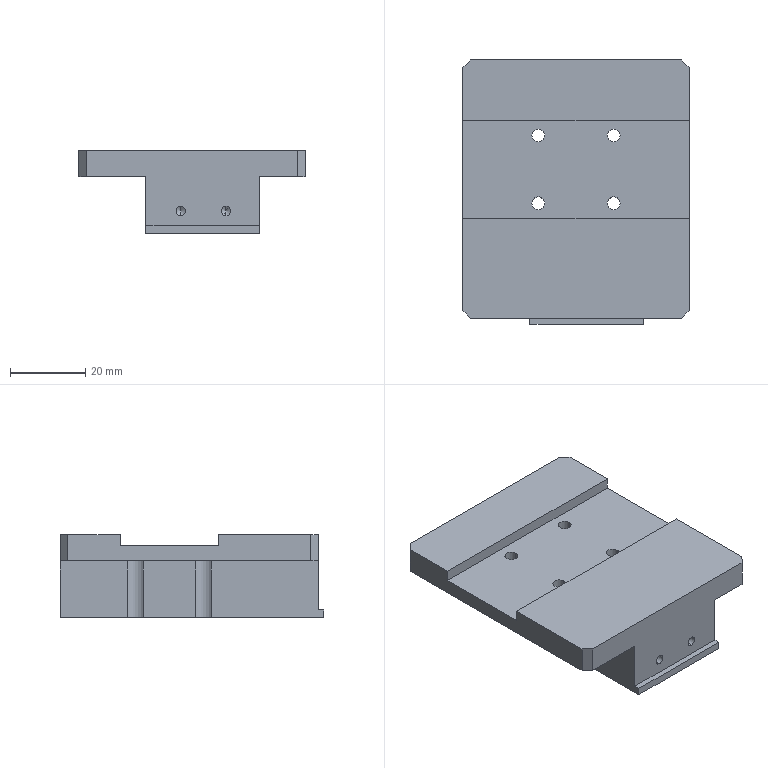Part | STEP file | 06-1040 module connection block | 1 solid | 62 faces | box 60 x 70 x 22 mm | volume 52388 mm3 | cylinder 26 | plane 24 | cone 12 | commonest cylinder face diameters 3.4 x8 4.2 x8 6 x6 2.5 x4